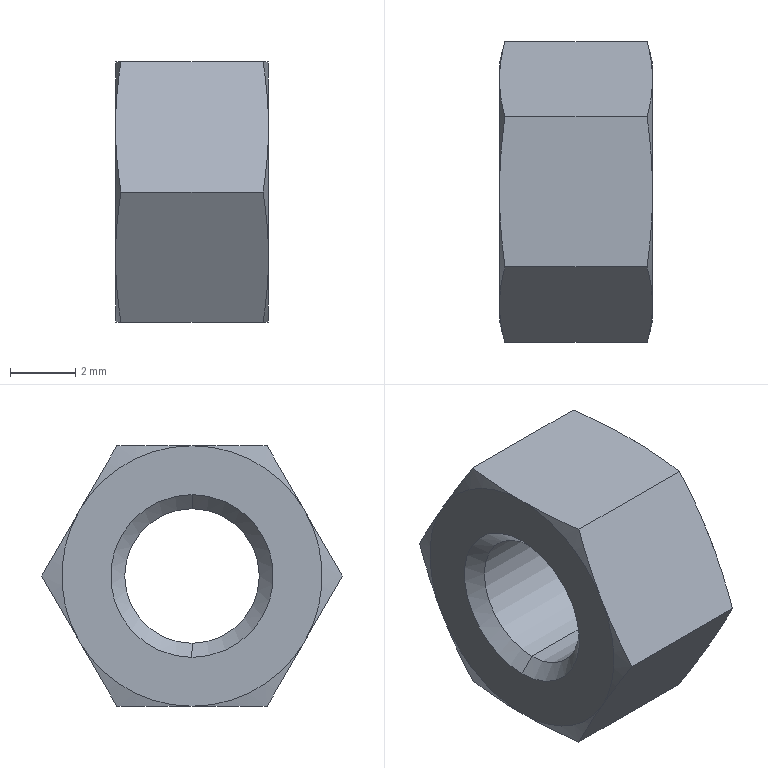Part | STEP file | QA-M5x0_8A | 1 solid | 26 faces | box 4.7 x 9.238 x 8 mm | volume 194.282 mm3 | cone 16 | plane 8 | cylinder 2 | commonest cylinder face diameters 4.134 x2